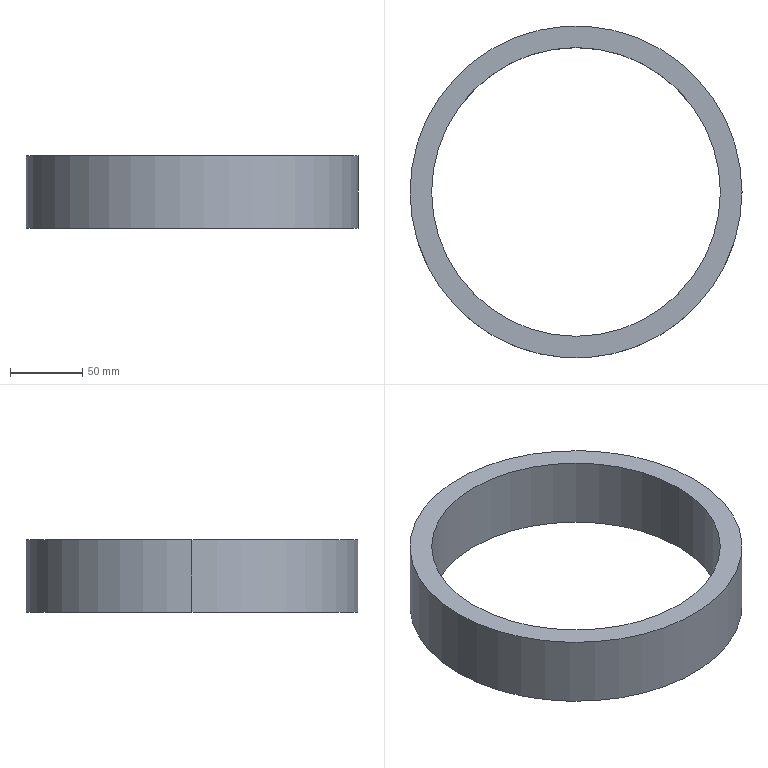Part | SolidWorks | features Extrusion 1 | 1 solid | 6 faces | box 230 x 230 x 50 mm | volume 506582 mm3 | cylinder 4 | plane 2 | commonest cylinder face diameters 200 x2 230 x2
STEP:
#1=CARTESIAN_POINT('',(-100.,0.,25.));
#2=VERTEX_POINT('',#1);
#3=CARTESIAN_POINT('',(100.,0.,25.));
#4=VERTEX_POINT('',#3);
#5=CARTESIAN_POINT('',(0.,0.,25.));
#6=DIRECTION('',(0.,0.,1.));
#7=DIRECTION('',(1.,0.,0.));
#8=AXIS2_PLACEMENT_3D('',#5,#6,#7);
#9=CIRCLE('',#8,100.);
#10=EDGE_CURVE('',#2,#4,#9,.T.);
#11=ORIENTED_EDGE('',*,*,#10,.T.);
#12=CARTESIAN_POINT('',(100.,0.,-25.));
#13=VERTEX_POINT('',#12);
#14=CARTESIAN_POINT('',(100.,0.,25.));
#15=DIRECTION('',(0.,0.,-1.));
#16=VECTOR('',#15,1000.);
#17=LINE('',#14,#16);
#18=EDGE_CURVE('',#4,#13,#17,.T.);
#19=ORIENTED_EDGE('',*,*,#18,.T.);
#20=CARTESIAN_POINT('',(-100.,0.,-25.));
#21=VERTEX_POINT('',#20);
#22=CARTESIAN_POINT('',(0.,0.,-25.));
#23=DIRECTION('',(0.,0.,1.));
#24=DIRECTION('',(1.,0.,0.));
#25=AXIS2_PLACEMENT_3D('',#22,#23,#24);
#26=CIRCLE('',#25,100.);
#27=EDGE_CURVE('',#21,#13,#26,.T.);
#28=ORIENTED_EDGE('',*,*,#27,.F.);
#29=CARTESIAN_POINT('',(-100.,0.,25.));
#30=DIRECTION('',(0.,0.,-1.));
#31=VECTOR('',#30,1000.);
#32=LINE('',#29,#31);
#33=EDGE_CURVE('',#2,#21,#32,.T.);
#34=ORIENTED_EDGE('',*,*,#33,.F.);
#35=EDGE_LOOP('',(#11,#19,#28,#34));
#36=FACE_OUTER_BOUND('',#35,.T.);
#37=CARTESIAN_POINT('',(0.,0.,25.));
#38=DIRECTION('',(0.,0.,-1.));
#39=DIRECTION('',(-1.,0.,0.));
#40=AXIS2_PLACEMENT_3D('',#37,#38,#39);
#41=CYLINDRICAL_SURFACE('',#40,100.);
#42=ADVANCED_FACE('',(#36),#41,.F.);
#43=CARTESIAN_POINT('',(115.,0.,25.));
#44=VERTEX_POINT('',#43);
#45=CARTESIAN_POINT('',(-115.,0.,25.));
#46=VERTEX_POINT('',#45);
#47=CARTESIAN_POINT('',(0.,0.,25.));
#48=DIRECTION('',(0.,0.,1.));
#49=DIRECTION('',(1.,0.,0.));
#50=AXIS2_PLACEMENT_3D('',#47,#48,#49);
#51=CIRCLE('',#50,115.);
#52=EDGE_CURVE('',#44,#46,#51,.T.);
#53=ORIENTED_EDGE('',*,*,#52,.F.);
#54=CARTESIAN_POINT('',(115.,0.,-25.));
#55=VERTEX_POINT('',#54);
#56=CARTESIAN_POINT('',(115.,0.,25.));
#57=DIRECTION('',(0.,0.,-1.));
#58=VECTOR('',#57,1000.);
#59=LINE('',#56,#58);
#60=EDGE_CURVE('',#44,#55,#59,.T.);
#61=ORIENTED_EDGE('',*,*,#60,.T.);
#62=CARTESIAN_POINT('',(-115.,0.,-25.));
#63=VERTEX_POINT('',#62);
#64=CARTESIAN_POINT('',(0.,0.,-25.));
#65=DIRECTION('',(0.,0.,1.));
#66=DIRECTION('',(1.,0.,0.));
#67=AXIS2_PLACEMENT_3D('',#64,#65,#66);
#68=CIRCLE('',#67,115.);
#69=EDGE_CURVE('',#55,#63,#68,.T.);
#70=ORIENTED_EDGE('',*,*,#69,.T.);
#71=CARTESIAN_POINT('',(-115.,0.,25.));
#72=DIRECTION('',(0.,0.,-1.));
#73=VECTOR('',#72,1000.);
#74=LINE('',#71,#73);
#75=EDGE_CURVE('',#46,#63,#74,.T.);
#76=ORIENTED_EDGE('',*,*,#75,.F.);
#77=EDGE_LOOP('',(#53,#61,#70,#76));
#78=FACE_OUTER_BOUND('',#77,.T.);
#79=CARTESIAN_POINT('',(0.,0.,25.));
#80=DIRECTION('',(0.,0.,-1.));
#81=DIRECTION('',(-1.,0.,0.));
#82=AXIS2_PLACEMENT_3D('',#79,#80,#81);
#83=CYLINDRICAL_SURFACE('',#82,115.);
#84=ADVANCED_FACE('',(#78),#83,.T.);
#85=CARTESIAN_POINT('',(0.,0.,25.));
#86=DIRECTION('',(0.,0.,1.));
#87=DIRECTION('',(1.,0.,0.));
#88=AXIS2_PLACEMENT_3D('',#85,#86,#87);
#89=CIRCLE('',#88,115.);
#90=EDGE_CURVE('',#46,#44,#89,.T.);
#91=ORIENTED_EDGE('',*,*,#90,.T.);
#92=ORIENTED_EDGE('',*,*,#52,.T.);
#93=EDGE_LOOP('',(#91,#92));
#94=FACE_OUTER_BOUND('',#93,.T.);
#95=ORIENTED_EDGE('',*,*,#10,.F.);
#96=CARTESIAN_POINT('',(0.,0.,25.));
#97=DIRECTION('',(0.,0.,1.));
#98=DIRECTION('',(1.,0.,0.));
#99=AXIS2_PLACEMENT_3D('',#96,#97,#98);
#100=CIRCLE('',#99,100.);
#101=EDGE_CURVE('',#4,#2,#100,.T.);
#102=ORIENTED_EDGE('',*,*,#101,.F.);
#103=EDGE_LOOP('',(#95,#102));
#104=FACE_BOUND('',#103,.T.);
#105=CARTESIAN_POINT('',(0.,0.,25.));
#106=DIRECTION('',(0.,0.,1.));
#107=DIRECTION('',(1.,0.,0.));
#108=AXIS2_PLACEMENT_3D('',#105,#106,#107);
#109=PLANE('',#108);
#110=ADVANCED_FACE('',(#94,#104),#109,.T.);
#111=CARTESIAN_POINT('',(0.,0.,-25.));
#112=DIRECTION('',(0.,0.,1.));
#113=DIRECTION('',(1.,0.,0.));
#114=AXIS2_PLACEMENT_3D('',#111,#112,#113);
#115=CIRCLE('',#114,115.);
#116=EDGE_CURVE('',#63,#55,#115,.T.);
#117=ORIENTED_EDGE('',*,*,#116,.F.);
#118=ORIENTED_EDGE('',*,*,#69,.F.);
#119=EDGE_LOOP('',(#117,#118));
#120=FACE_OUTER_BOUND('',#119,.T.);
#121=ORIENTED_EDGE('',*,*,#27,.T.);
#122=CARTESIAN_POINT('',(0.,0.,-25.));
#123=DIRECTION('',(0.,0.,1.));
#124=DIRECTION('',(1.,0.,0.));
#125=AXIS2_PLACEMENT_3D('',#122,#123,#124);
#126=CIRCLE('',#125,100.);
#127=EDGE_CURVE('',#13,#21,#126,.T.);
#128=ORIENTED_EDGE('',*,*,#127,.T.);
#129=EDGE_LOOP('',(#121,#128));
#130=FACE_BOUND('',#129,.T.);
#131=CARTESIAN_POINT('',(0.,0.,-25.));
#132=DIRECTION('',(0.,0.,1.));
#133=DIRECTION('',(1.,0.,0.));
#134=AXIS2_PLACEMENT_3D('',#131,#132,#133);
#135=PLANE('',#134);
#136=ADVANCED_FACE('',(#120,#130),#135,.F.);
#137=ORIENTED_EDGE('',*,*,#60,.F.);
#138=ORIENTED_EDGE('',*,*,#90,.F.);
#139=ORIENTED_EDGE('',*,*,#75,.T.);
#140=ORIENTED_EDGE('',*,*,#116,.T.);
#141=EDGE_LOOP('',(#137,#138,#139,#140));
#142=FACE_OUTER_BOUND('',#141,.T.);
#143=CARTESIAN_POINT('',(0.,0.,25.));
#144=DIRECTION('',(0.,0.,-1.));
#145=DIRECTION('',(-1.,0.,0.));
#146=AXIS2_PLACEMENT_3D('',#143,#144,#145);
#147=CYLINDRICAL_SURFACE('',#146,115.);
#148=ADVANCED_FACE('',(#142),#147,.T.);
#149=ORIENTED_EDGE('',*,*,#18,.F.);
#150=ORIENTED_EDGE('',*,*,#101,.T.);
#151=ORIENTED_EDGE('',*,*,#33,.T.);
#152=ORIENTED_EDGE('',*,*,#127,.F.);
#153=EDGE_LOOP('',(#149,#150,#151,#152));
#154=FACE_OUTER_BOUND('',#153,.T.);
#155=CARTESIAN_POINT('',(0.,0.,25.));
#156=DIRECTION('',(0.,0.,-1.));
#157=DIRECTION('',(-1.,0.,0.));
#158=AXIS2_PLACEMENT_3D('',#155,#156,#157);
#159=CYLINDRICAL_SURFACE('',#158,100.);
#160=ADVANCED_FACE('',(#154),#159,.F.);
#161=CLOSED_SHELL('',(#42,#84,#110,#136,#148,#160));
#162=MANIFOLD_SOLID_BREP('',#161);
#163=CARTESIAN_POINT('',(0.,0.,0.));
#164=DIRECTION('',(0.,0.,1.));
#165=DIRECTION('',(1.,0.,0.));
#166=AXIS2_PLACEMENT_3D('',#163,#164,#165);
#167=(LENGTH_UNIT()NAMED_UNIT(*)SI_UNIT(.MILLI.,.METRE.));
#168=UNCERTAINTY_MEASURE_WITH_UNIT(LENGTH_MEASURE(0.00001),#167,'','');
#169=(NAMED_UNIT(*)PLANE_ANGLE_UNIT()SI_UNIT($,.RADIAN.));
#170=(NAMED_UNIT(*)SI_UNIT($,.STERADIAN.)SOLID_ANGLE_UNIT());
#171=(GEOMETRIC_REPRESENTATION_CONTEXT(3)GLOBAL_UNCERTAINTY_ASSIGNED_CONTEXT((#168))GLOBAL_UNIT_ASSIGNED_CONTEXT((#167,#169,#170))REPRESENTATION_CONTEXT('',''));
#172=ADVANCED_BREP_SHAPE_REPRESENTATION('',(#162,#166),#171);